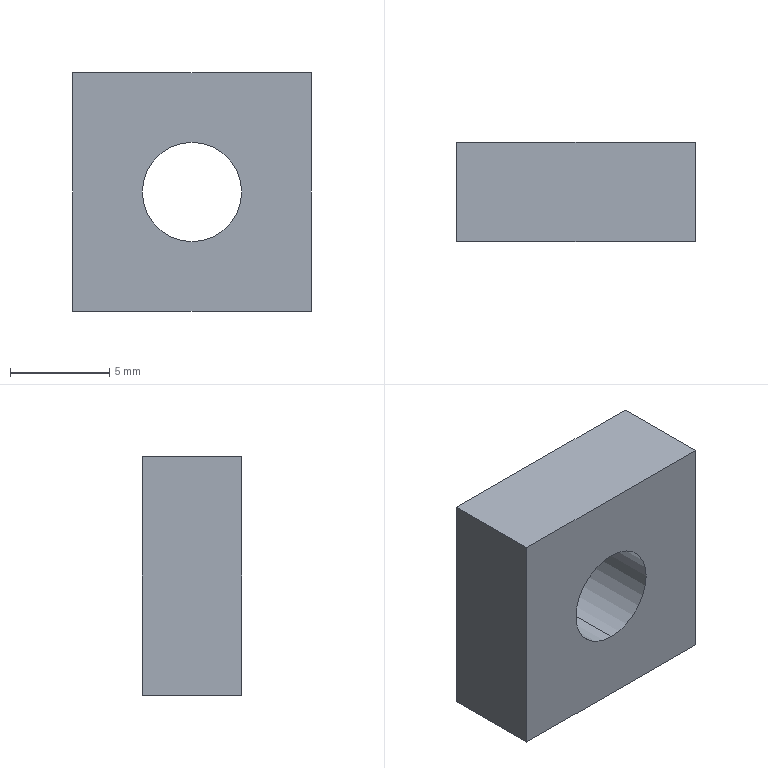Part | SolidWorks | features FlatPattern 1, HoleWzd 1, SMBaseFlange 1, SheetMetal 1 | 1 solid | 8 faces | box 12 x 5 x 12 mm | volume 621.825 mm3 | plane 6 | cylinder 2 | commonest cylinder face diameters 5 x2
STEP:
#1=CARTESIAN_POINT('',(0.,0.,-2.5));
#2=VERTEX_POINT('',#1);
#3=CARTESIAN_POINT('',(0.,0.,2.5));
#4=VERTEX_POINT('',#3);
#5=CARTESIAN_POINT('',(0.,0.,0.));
#6=DIRECTION('',(0.,1.,0.));
#7=DIRECTION('',(0.,0.,1.));
#8=AXIS2_PLACEMENT_3D('',#5,#6,#7);
#9=CIRCLE('',#8,2.5);
#10=EDGE_CURVE('',#2,#4,#9,.T.);
#11=ORIENTED_EDGE('',*,*,#10,.F.);
#12=CARTESIAN_POINT('',(0.,5.,-2.5));
#13=VERTEX_POINT('',#12);
#14=CARTESIAN_POINT('',(0.,5.,-2.5));
#15=DIRECTION('',(0.,1.,0.));
#16=VECTOR('',#15,1000.);
#17=LINE('',#14,#16);
#18=EDGE_CURVE('',#2,#13,#17,.T.);
#19=ORIENTED_EDGE('',*,*,#18,.T.);
#20=CARTESIAN_POINT('',(0.,5.,2.5));
#21=VERTEX_POINT('',#20);
#22=CARTESIAN_POINT('',(0.,5.,0.));
#23=DIRECTION('',(0.,1.,0.));
#24=DIRECTION('',(0.,0.,1.));
#25=AXIS2_PLACEMENT_3D('',#22,#23,#24);
#26=CIRCLE('',#25,2.5);
#27=EDGE_CURVE('',#13,#21,#26,.T.);
#28=ORIENTED_EDGE('',*,*,#27,.T.);
#29=CARTESIAN_POINT('',(0.,5.,2.5));
#30=DIRECTION('',(0.,1.,0.));
#31=VECTOR('',#30,1000.);
#32=LINE('',#29,#31);
#33=EDGE_CURVE('',#4,#21,#32,.T.);
#34=ORIENTED_EDGE('',*,*,#33,.F.);
#35=EDGE_LOOP('',(#11,#19,#28,#34));
#36=FACE_OUTER_BOUND('',#35,.T.);
#37=CARTESIAN_POINT('',(0.,5.,0.));
#38=DIRECTION('',(0.,1.,0.));
#39=DIRECTION('',(0.,0.,1.));
#40=AXIS2_PLACEMENT_3D('',#37,#38,#39);
#41=CYLINDRICAL_SURFACE('',#40,2.5);
#42=ADVANCED_FACE('',(#36),#41,.F.);
#43=CARTESIAN_POINT('',(6.,0.,6.));
#44=VERTEX_POINT('',#43);
#45=CARTESIAN_POINT('',(6.,0.,-6.));
#46=VERTEX_POINT('',#45);
#47=CARTESIAN_POINT('',(6.,0.,-6.));
#48=DIRECTION('',(0.,0.,-1.));
#49=VECTOR('',#48,1000.);
#50=LINE('',#47,#49);
#51=EDGE_CURVE('',#44,#46,#50,.T.);
#52=ORIENTED_EDGE('',*,*,#51,.T.);
#53=CARTESIAN_POINT('',(6.,5.,-6.));
#54=VERTEX_POINT('',#53);
#55=CARTESIAN_POINT('',(6.,5.,-6.));
#56=DIRECTION('',(0.,-1.,0.));
#57=VECTOR('',#56,1000.);
#58=LINE('',#55,#57);
#59=EDGE_CURVE('',#54,#46,#58,.T.);
#60=ORIENTED_EDGE('',*,*,#59,.F.);
#61=CARTESIAN_POINT('',(6.,5.,6.));
#62=VERTEX_POINT('',#61);
#63=CARTESIAN_POINT('',(6.,5.,-6.));
#64=DIRECTION('',(0.,0.,-1.));
#65=VECTOR('',#64,1000.);
#66=LINE('',#63,#65);
#67=EDGE_CURVE('',#62,#54,#66,.T.);
#68=ORIENTED_EDGE('',*,*,#67,.F.);
#69=CARTESIAN_POINT('',(6.,5.,6.));
#70=DIRECTION('',(0.,-1.,0.));
#71=VECTOR('',#70,1000.);
#72=LINE('',#69,#71);
#73=EDGE_CURVE('',#62,#44,#72,.T.);
#74=ORIENTED_EDGE('',*,*,#73,.T.);
#75=EDGE_LOOP('',(#52,#60,#68,#74));
#76=FACE_OUTER_BOUND('',#75,.T.);
#77=CARTESIAN_POINT('',(6.,5.,-6.));
#78=DIRECTION('',(-1.,0.,0.));
#79=DIRECTION('',(0.,0.,1.));
#80=AXIS2_PLACEMENT_3D('',#77,#78,#79);
#81=PLANE('',#80);
#82=ADVANCED_FACE('',(#76),#81,.F.);
#83=CARTESIAN_POINT('',(-6.,0.,-6.));
#84=VERTEX_POINT('',#83);
#85=CARTESIAN_POINT('',(-6.,0.,-6.));
#86=DIRECTION('',(-1.,0.,0.));
#87=VECTOR('',#86,1000.);
#88=LINE('',#85,#87);
#89=EDGE_CURVE('',#46,#84,#88,.T.);
#90=ORIENTED_EDGE('',*,*,#89,.T.);
#91=CARTESIAN_POINT('',(-6.,5.,-6.));
#92=VERTEX_POINT('',#91);
#93=CARTESIAN_POINT('',(-6.,5.,-6.));
#94=DIRECTION('',(0.,-1.,0.));
#95=VECTOR('',#94,1000.);
#96=LINE('',#93,#95);
#97=EDGE_CURVE('',#92,#84,#96,.T.);
#98=ORIENTED_EDGE('',*,*,#97,.F.);
#99=CARTESIAN_POINT('',(-6.,5.,-6.));
#100=DIRECTION('',(-1.,0.,0.));
#101=VECTOR('',#100,1000.);
#102=LINE('',#99,#101);
#103=EDGE_CURVE('',#54,#92,#102,.T.);
#104=ORIENTED_EDGE('',*,*,#103,.F.);
#105=ORIENTED_EDGE('',*,*,#59,.T.);
#106=EDGE_LOOP('',(#90,#98,#104,#105));
#107=FACE_OUTER_BOUND('',#106,.T.);
#108=CARTESIAN_POINT('',(-6.,5.,-6.));
#109=DIRECTION('',(0.,0.,1.));
#110=DIRECTION('',(1.,0.,0.));
#111=AXIS2_PLACEMENT_3D('',#108,#109,#110);
#112=PLANE('',#111);
#113=ADVANCED_FACE('',(#107),#112,.F.);
#114=CARTESIAN_POINT('',(-6.,0.,6.));
#115=VERTEX_POINT('',#114);
#116=CARTESIAN_POINT('',(-6.,0.,-6.));
#117=DIRECTION('',(0.,0.,1.));
#118=VECTOR('',#117,1000.);
#119=LINE('',#116,#118);
#120=EDGE_CURVE('',#84,#115,#119,.T.);
#121=ORIENTED_EDGE('',*,*,#120,.T.);
#122=CARTESIAN_POINT('',(-6.,5.,6.));
#123=VERTEX_POINT('',#122);
#124=CARTESIAN_POINT('',(-6.,5.,6.));
#125=DIRECTION('',(0.,-1.,0.));
#126=VECTOR('',#125,1000.);
#127=LINE('',#124,#126);
#128=EDGE_CURVE('',#123,#115,#127,.T.);
#129=ORIENTED_EDGE('',*,*,#128,.F.);
#130=CARTESIAN_POINT('',(-6.,5.,-6.));
#131=DIRECTION('',(0.,0.,1.));
#132=VECTOR('',#131,1000.);
#133=LINE('',#130,#132);
#134=EDGE_CURVE('',#92,#123,#133,.T.);
#135=ORIENTED_EDGE('',*,*,#134,.F.);
#136=ORIENTED_EDGE('',*,*,#97,.T.);
#137=EDGE_LOOP('',(#121,#129,#135,#136));
#138=FACE_OUTER_BOUND('',#137,.T.);
#139=CARTESIAN_POINT('',(-6.,5.,-6.));
#140=DIRECTION('',(1.,0.,0.));
#141=DIRECTION('',(0.,0.,-1.));
#142=AXIS2_PLACEMENT_3D('',#139,#140,#141);
#143=PLANE('',#142);
#144=ADVANCED_FACE('',(#138),#143,.F.);
#145=CARTESIAN_POINT('',(-6.,0.,6.));
#146=DIRECTION('',(1.,0.,0.));
#147=VECTOR('',#146,1000.);
#148=LINE('',#145,#147);
#149=EDGE_CURVE('',#115,#44,#148,.T.);
#150=ORIENTED_EDGE('',*,*,#149,.T.);
#151=ORIENTED_EDGE('',*,*,#73,.F.);
#152=CARTESIAN_POINT('',(-6.,5.,6.));
#153=DIRECTION('',(1.,0.,0.));
#154=VECTOR('',#153,1000.);
#155=LINE('',#152,#154);
#156=EDGE_CURVE('',#123,#62,#155,.T.);
#157=ORIENTED_EDGE('',*,*,#156,.F.);
#158=ORIENTED_EDGE('',*,*,#128,.T.);
#159=EDGE_LOOP('',(#150,#151,#157,#158));
#160=FACE_OUTER_BOUND('',#159,.T.);
#161=CARTESIAN_POINT('',(-6.,5.,6.));
#162=DIRECTION('',(0.,0.,-1.));
#163=DIRECTION('',(-1.,0.,0.));
#164=AXIS2_PLACEMENT_3D('',#161,#162,#163);
#165=PLANE('',#164);
#166=ADVANCED_FACE('',(#160),#165,.F.);
#167=CARTESIAN_POINT('',(0.,5.,0.));
#168=DIRECTION('',(0.,1.,0.));
#169=DIRECTION('',(0.,0.,1.));
#170=AXIS2_PLACEMENT_3D('',#167,#168,#169);
#171=CIRCLE('',#170,2.5);
#172=EDGE_CURVE('',#21,#13,#171,.T.);
#173=ORIENTED_EDGE('',*,*,#172,.F.);
#174=ORIENTED_EDGE('',*,*,#27,.F.);
#175=EDGE_LOOP('',(#173,#174));
#176=FACE_BOUND('',#175,.T.);
#177=ORIENTED_EDGE('',*,*,#67,.T.);
#178=ORIENTED_EDGE('',*,*,#103,.T.);
#179=ORIENTED_EDGE('',*,*,#134,.T.);
#180=ORIENTED_EDGE('',*,*,#156,.T.);
#181=EDGE_LOOP('',(#177,#178,#179,#180));
#182=FACE_OUTER_BOUND('',#181,.T.);
#183=CARTESIAN_POINT('',(0.,5.,0.));
#184=DIRECTION('',(0.,1.,0.));
#185=DIRECTION('',(0.,0.,1.));
#186=AXIS2_PLACEMENT_3D('',#183,#184,#185);
#187=PLANE('',#186);
#188=ADVANCED_FACE('',(#176,#182),#187,.T.);
#189=CARTESIAN_POINT('',(0.,0.,0.));
#190=DIRECTION('',(0.,1.,0.));
#191=DIRECTION('',(0.,0.,1.));
#192=AXIS2_PLACEMENT_3D('',#189,#190,#191);
#193=CIRCLE('',#192,2.5);
#194=EDGE_CURVE('',#4,#2,#193,.T.);
#195=ORIENTED_EDGE('',*,*,#194,.T.);
#196=ORIENTED_EDGE('',*,*,#10,.T.);
#197=EDGE_LOOP('',(#195,#196));
#198=FACE_BOUND('',#197,.T.);
#199=ORIENTED_EDGE('',*,*,#51,.F.);
#200=ORIENTED_EDGE('',*,*,#149,.F.);
#201=ORIENTED_EDGE('',*,*,#120,.F.);
#202=ORIENTED_EDGE('',*,*,#89,.F.);
#203=EDGE_LOOP('',(#199,#200,#201,#202));
#204=FACE_OUTER_BOUND('',#203,.T.);
#205=CARTESIAN_POINT('',(0.,0.,0.));
#206=DIRECTION('',(0.,1.,0.));
#207=DIRECTION('',(0.,0.,1.));
#208=AXIS2_PLACEMENT_3D('',#205,#206,#207);
#209=PLANE('',#208);
#210=ADVANCED_FACE('',(#198,#204),#209,.F.);
#211=ORIENTED_EDGE('',*,*,#18,.F.);
#212=ORIENTED_EDGE('',*,*,#194,.F.);
#213=ORIENTED_EDGE('',*,*,#33,.T.);
#214=ORIENTED_EDGE('',*,*,#172,.T.);
#215=EDGE_LOOP('',(#211,#212,#213,#214));
#216=FACE_OUTER_BOUND('',#215,.T.);
#217=CARTESIAN_POINT('',(0.,5.,0.));
#218=DIRECTION('',(0.,1.,0.));
#219=DIRECTION('',(0.,0.,1.));
#220=AXIS2_PLACEMENT_3D('',#217,#218,#219);
#221=CYLINDRICAL_SURFACE('',#220,2.5);
#222=ADVANCED_FACE('',(#216),#221,.F.);
#223=CLOSED_SHELL('',(#42,#82,#113,#144,#166,#188,#210,#222));
#224=MANIFOLD_SOLID_BREP('',#223);
#225=CARTESIAN_POINT('',(0.,0.,0.));
#226=DIRECTION('',(0.,0.,1.));
#227=DIRECTION('',(1.,0.,0.));
#228=AXIS2_PLACEMENT_3D('',#225,#226,#227);
#229=(LENGTH_UNIT()NAMED_UNIT(*)SI_UNIT(.MILLI.,.METRE.));
#230=UNCERTAINTY_MEASURE_WITH_UNIT(LENGTH_MEASURE(0.00001),#229,'','');
#231=(NAMED_UNIT(*)PLANE_ANGLE_UNIT()SI_UNIT($,.RADIAN.));
#232=(NAMED_UNIT(*)SI_UNIT($,.STERADIAN.)SOLID_ANGLE_UNIT());
#233=(GEOMETRIC_REPRESENTATION_CONTEXT(3)GLOBAL_UNCERTAINTY_ASSIGNED_CONTEXT((#230))GLOBAL_UNIT_ASSIGNED_CONTEXT((#229,#231,#232))REPRESENTATION_CONTEXT('',''));
#234=ADVANCED_BREP_SHAPE_REPRESENTATION('',(#224,#228),#233);